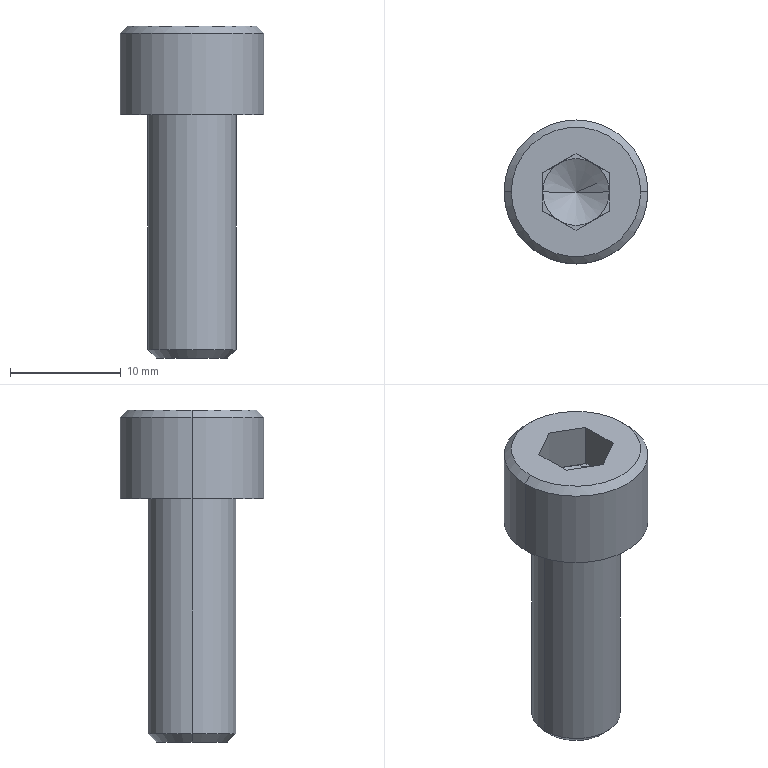Part | NX | features BREP 1 | 1 solid | 25 faces | box 13 x 13 x 30 mm | volume 2011 mm3 | plane 15 | cone 6 | cylinder 4 | commonest cylinder face diameters 8 x2 13 x2
STEP:
#1=CARTESIAN_POINT('',(0.,0.,2.268));
#2=VERTEX_POINT('',#1);
#3=CARTESIAN_POINT('',(3.,0.,4.));
#4=VERTEX_POINT('',#3);
#5=CARTESIAN_POINT('',(0.,0.,2.268));
#6=DIRECTION('',(0.866,0.,0.5));
#7=VECTOR('',#6,1000.);
#8=LINE('',#5,#7);
#9=EDGE_CURVE('',#2,#4,#8,.T.);
#10=ORIENTED_EDGE('',*,*,#9,.F.);
#11=CARTESIAN_POINT('',(-3.,0.,4.));
#12=VERTEX_POINT('',#11);
#13=CARTESIAN_POINT('',(0.,0.,2.268));
#14=DIRECTION('',(-0.866,0.,0.5));
#15=VECTOR('',#14,1000.);
#16=LINE('',#13,#15);
#17=EDGE_CURVE('',#2,#12,#16,.T.);
#18=ORIENTED_EDGE('',*,*,#17,.T.);
#19=CARTESIAN_POINT('',(-1.5,-2.598,4.));
#20=VERTEX_POINT('',#19);
#21=CARTESIAN_POINT('',(0.,0.,4.));
#22=DIRECTION('',(0.,0.,1.));
#23=DIRECTION('',(1.,0.,0.));
#24=AXIS2_PLACEMENT_3D('',#21,#22,#23);
#25=CIRCLE('',#24,3.);
#26=EDGE_CURVE('',#12,#20,#25,.T.);
#27=ORIENTED_EDGE('',*,*,#26,.T.);
#28=CARTESIAN_POINT('',(1.5,-2.598,4.));
#29=VERTEX_POINT('',#28);
#30=CARTESIAN_POINT('',(0.,0.,4.));
#31=DIRECTION('',(0.,0.,1.));
#32=DIRECTION('',(1.,0.,0.));
#33=AXIS2_PLACEMENT_3D('',#30,#31,#32);
#34=CIRCLE('',#33,3.);
#35=EDGE_CURVE('',#20,#29,#34,.T.);
#36=ORIENTED_EDGE('',*,*,#35,.T.);
#37=CARTESIAN_POINT('',(0.,0.,4.));
#38=DIRECTION('',(0.,0.,1.));
#39=DIRECTION('',(1.,0.,0.));
#40=AXIS2_PLACEMENT_3D('',#37,#38,#39);
#41=CIRCLE('',#40,3.);
#42=EDGE_CURVE('',#29,#4,#41,.T.);
#43=ORIENTED_EDGE('',*,*,#42,.T.);
#44=EDGE_LOOP('',(#10,#18,#27,#36,#43));
#45=FACE_BOUND('',#44,.T.);
#46=CARTESIAN_POINT('',(0.,0.,1002.268));
#47=DIRECTION('',(0.,0.,1.));
#48=DIRECTION('',(-1.,0.,0.));
#49=AXIS2_PLACEMENT_3D('',#46,#47,#48);
#50=CONICAL_SURFACE('',#49,1732.051,1.047);
#51=ADVANCED_FACE('',(#45),#50,.F.);
#52=CARTESIAN_POINT('',(6.5,0.,0.));
#53=VERTEX_POINT('',#52);
#54=CARTESIAN_POINT('',(-6.5,0.,0.));
#55=VERTEX_POINT('',#54);
#56=CARTESIAN_POINT('',(0.,0.,0.));
#57=DIRECTION('',(0.,0.,1.));
#58=DIRECTION('',(1.,0.,0.));
#59=AXIS2_PLACEMENT_3D('',#56,#57,#58);
#60=CIRCLE('',#59,6.5);
#61=EDGE_CURVE('',#53,#55,#60,.T.);
#62=ORIENTED_EDGE('',*,*,#61,.T.);
#63=CARTESIAN_POINT('',(-6.5,0.,7.35));
#64=VERTEX_POINT('',#63);
#65=CARTESIAN_POINT('',(-6.5,0.,0.));
#66=DIRECTION('',(0.,0.,1.));
#67=VECTOR('',#66,1000.);
#68=LINE('',#65,#67);
#69=EDGE_CURVE('',#55,#64,#68,.T.);
#70=ORIENTED_EDGE('',*,*,#69,.T.);
#71=CARTESIAN_POINT('',(6.5,0.,7.35));
#72=VERTEX_POINT('',#71);
#73=CARTESIAN_POINT('',(0.,0.,7.35));
#74=DIRECTION('',(0.,0.,1.));
#75=DIRECTION('',(1.,0.,0.));
#76=AXIS2_PLACEMENT_3D('',#73,#74,#75);
#77=CIRCLE('',#76,6.5);
#78=EDGE_CURVE('',#72,#64,#77,.T.);
#79=ORIENTED_EDGE('',*,*,#78,.F.);
#80=CARTESIAN_POINT('',(6.5,0.,0.));
#81=DIRECTION('',(0.,0.,1.));
#82=VECTOR('',#81,1000.);
#83=LINE('',#80,#82);
#84=EDGE_CURVE('',#53,#72,#83,.T.);
#85=ORIENTED_EDGE('',*,*,#84,.F.);
#86=EDGE_LOOP('',(#62,#70,#79,#85));
#87=FACE_BOUND('',#86,.T.);
#88=CARTESIAN_POINT('',(0.,0.,0.));
#89=DIRECTION('',(0.,0.,1.));
#90=DIRECTION('',(-1.,0.,0.));
#91=AXIS2_PLACEMENT_3D('',#88,#89,#90);
#92=CYLINDRICAL_SURFACE('',#91,6.5);
#93=ADVANCED_FACE('',(#87),#92,.T.);
#94=CARTESIAN_POINT('',(5.85,0.,8.));
#95=VERTEX_POINT('',#94);
#96=CARTESIAN_POINT('',(-5.85,0.,8.));
#97=VERTEX_POINT('',#96);
#98=CARTESIAN_POINT('',(0.,0.,8.));
#99=DIRECTION('',(0.,0.,1.));
#100=DIRECTION('',(1.,0.,0.));
#101=AXIS2_PLACEMENT_3D('',#98,#99,#100);
#102=CIRCLE('',#101,5.85);
#103=EDGE_CURVE('',#95,#97,#102,.T.);
#104=ORIENTED_EDGE('',*,*,#103,.F.);
#105=CARTESIAN_POINT('',(6.5,0.,7.35));
#106=DIRECTION('',(0.7071,0.,-0.7071));
#107=VECTOR('',#106,1000.);
#108=LINE('',#105,#107);
#109=EDGE_CURVE('',#72,#95,#108,.F.);
#110=ORIENTED_EDGE('',*,*,#109,.F.);
#111=ORIENTED_EDGE('',*,*,#78,.T.);
#112=CARTESIAN_POINT('',(-6.5,0.,7.35));
#113=DIRECTION('',(-0.7071,0.,-0.7071));
#114=VECTOR('',#113,1000.);
#115=LINE('',#112,#114);
#116=EDGE_CURVE('',#64,#97,#115,.F.);
#117=ORIENTED_EDGE('',*,*,#116,.T.);
#118=EDGE_LOOP('',(#104,#110,#111,#117));
#119=FACE_BOUND('',#118,.T.);
#120=CARTESIAN_POINT('',(0.,0.,7.35));
#121=DIRECTION('',(0.,0.,-1.));
#122=DIRECTION('',(1.,0.,0.));
#123=AXIS2_PLACEMENT_3D('',#120,#121,#122);
#124=CONICAL_SURFACE('',#123,6.5,0.7854);
#125=ADVANCED_FACE('',(#119),#124,.T.);
#126=CARTESIAN_POINT('',(3.233,0.,-22.));
#127=VERTEX_POINT('',#126);
#128=CARTESIAN_POINT('',(-3.233,0.,-22.));
#129=VERTEX_POINT('',#128);
#130=CARTESIAN_POINT('',(0.,0.,-22.));
#131=DIRECTION('',(0.,0.,1.));
#132=DIRECTION('',(1.,0.,0.));
#133=AXIS2_PLACEMENT_3D('',#130,#131,#132);
#134=CIRCLE('',#133,3.233);
#135=EDGE_CURVE('',#127,#129,#134,.T.);
#136=ORIENTED_EDGE('',*,*,#135,.T.);
#137=CARTESIAN_POINT('',(-4.,0.,-21.233));
#138=VERTEX_POINT('',#137);
#139=CARTESIAN_POINT('',(-3.233,0.,-22.));
#140=DIRECTION('',(-0.7071,0.,0.7071));
#141=VECTOR('',#140,1000.);
#142=LINE('',#139,#141);
#143=EDGE_CURVE('',#129,#138,#142,.T.);
#144=ORIENTED_EDGE('',*,*,#143,.T.);
#145=CARTESIAN_POINT('',(4.,0.,-21.233));
#146=VERTEX_POINT('',#145);
#147=CARTESIAN_POINT('',(0.,0.,-21.233));
#148=DIRECTION('',(0.,0.,1.));
#149=DIRECTION('',(1.,0.,0.));
#150=AXIS2_PLACEMENT_3D('',#147,#148,#149);
#151=CIRCLE('',#150,4.);
#152=EDGE_CURVE('',#146,#138,#151,.T.);
#153=ORIENTED_EDGE('',*,*,#152,.F.);
#154=CARTESIAN_POINT('',(3.233,0.,-22.));
#155=DIRECTION('',(0.7071,0.,0.7071));
#156=VECTOR('',#155,1000.);
#157=LINE('',#154,#156);
#158=EDGE_CURVE('',#127,#146,#157,.T.);
#159=ORIENTED_EDGE('',*,*,#158,.F.);
#160=EDGE_LOOP('',(#136,#144,#153,#159));
#161=FACE_BOUND('',#160,.T.);
#162=CARTESIAN_POINT('',(0.,0.,-22.));
#163=DIRECTION('',(0.,0.,1.));
#164=DIRECTION('',(-1.,0.,0.));
#165=AXIS2_PLACEMENT_3D('',#162,#163,#164);
#166=CONICAL_SURFACE('',#165,3.233,0.7854);
#167=ADVANCED_FACE('',(#161),#166,.T.);
#168=ORIENTED_EDGE('',*,*,#152,.T.);
#169=CARTESIAN_POINT('',(-4.,0.,0.));
#170=VERTEX_POINT('',#169);
#171=CARTESIAN_POINT('',(-4.,0.,-22.));
#172=DIRECTION('',(0.,0.,1.));
#173=VECTOR('',#172,1000.);
#174=LINE('',#171,#173);
#175=EDGE_CURVE('',#138,#170,#174,.T.);
#176=ORIENTED_EDGE('',*,*,#175,.T.);
#177=CARTESIAN_POINT('',(4.,0.,0.));
#178=VERTEX_POINT('',#177);
#179=CARTESIAN_POINT('',(0.,0.,0.));
#180=DIRECTION('',(0.,0.,1.));
#181=DIRECTION('',(1.,0.,0.));
#182=AXIS2_PLACEMENT_3D('',#179,#180,#181);
#183=CIRCLE('',#182,4.);
#184=EDGE_CURVE('',#178,#170,#183,.T.);
#185=ORIENTED_EDGE('',*,*,#184,.F.);
#186=CARTESIAN_POINT('',(4.,0.,-22.));
#187=DIRECTION('',(0.,0.,1.));
#188=VECTOR('',#187,1000.);
#189=LINE('',#186,#188);
#190=EDGE_CURVE('',#146,#178,#189,.T.);
#191=ORIENTED_EDGE('',*,*,#190,.F.);
#192=EDGE_LOOP('',(#168,#176,#185,#191));
#193=FACE_BOUND('',#192,.T.);
#194=CARTESIAN_POINT('',(0.,0.,-22.));
#195=DIRECTION('',(0.,0.,1.));
#196=DIRECTION('',(-1.,0.,0.));
#197=AXIS2_PLACEMENT_3D('',#194,#195,#196);
#198=CYLINDRICAL_SURFACE('',#197,4.);
#199=ADVANCED_FACE('',(#193),#198,.T.);
#200=CARTESIAN_POINT('',(1.5,2.598,4.));
#201=VERTEX_POINT('',#200);
#202=CARTESIAN_POINT('',(0.,0.,4.));
#203=DIRECTION('',(0.,0.,1.));
#204=DIRECTION('',(1.,0.,0.));
#205=AXIS2_PLACEMENT_3D('',#202,#203,#204);
#206=CIRCLE('',#205,3.);
#207=EDGE_CURVE('',#4,#201,#206,.T.);
#208=ORIENTED_EDGE('',*,*,#207,.F.);
#209=CARTESIAN_POINT('',(3.,1.732,4.));
#210=VERTEX_POINT('',#209);
#211=CARTESIAN_POINT('',(3.,-1.732,4.));
#212=DIRECTION('',(0.,1.,0.));
#213=VECTOR('',#212,1000.);
#214=LINE('',#211,#213);
#215=EDGE_CURVE('',#4,#210,#214,.T.);
#216=ORIENTED_EDGE('',*,*,#215,.T.);
#217=CARTESIAN_POINT('',(3.,1.732,4.));
#218=DIRECTION('',(-0.866,0.5,0.));
#219=VECTOR('',#218,1000.);
#220=LINE('',#217,#219);
#221=EDGE_CURVE('',#210,#201,#220,.T.);
#222=ORIENTED_EDGE('',*,*,#221,.T.);
#223=EDGE_LOOP('',(#208,#216,#222));
#224=FACE_BOUND('',#223,.T.);
#225=CARTESIAN_POINT('',(0.,0.,4.));
#226=DIRECTION('',(0.,0.,1.));
#227=DIRECTION('',(-1.,0.,0.));
#228=AXIS2_PLACEMENT_3D('',#225,#226,#227);
#229=PLANE('',#228);
#230=ADVANCED_FACE('',(#224),#229,.T.);
#231=CARTESIAN_POINT('',(-1.5,2.598,4.));
#232=VERTEX_POINT('',#231);
#233=CARTESIAN_POINT('',(0.,0.,4.));
#234=DIRECTION('',(0.,0.,1.));
#235=DIRECTION('',(1.,0.,0.));
#236=AXIS2_PLACEMENT_3D('',#233,#234,#235);
#237=CIRCLE('',#236,3.);
#238=EDGE_CURVE('',#201,#232,#237,.T.);
#239=ORIENTED_EDGE('',*,*,#238,.F.);
#240=CARTESIAN_POINT('',(0.,3.464,4.));
#241=VERTEX_POINT('',#240);
#242=CARTESIAN_POINT('',(3.,1.732,4.));
#243=DIRECTION('',(-0.866,0.5,0.));
#244=VECTOR('',#243,1000.);
#245=LINE('',#242,#244);
#246=EDGE_CURVE('',#201,#241,#245,.T.);
#247=ORIENTED_EDGE('',*,*,#246,.T.);
#248=CARTESIAN_POINT('',(0.,3.464,4.));
#249=DIRECTION('',(-0.866,-0.5,0.));
#250=VECTOR('',#249,1000.);
#251=LINE('',#248,#250);
#252=EDGE_CURVE('',#241,#232,#251,.T.);
#253=ORIENTED_EDGE('',*,*,#252,.T.);
#254=EDGE_LOOP('',(#239,#247,#253));
#255=FACE_BOUND('',#254,.T.);
#256=CARTESIAN_POINT('',(0.,0.,4.));
#257=DIRECTION('',(0.,0.,1.));
#258=DIRECTION('',(-1.,0.,0.));
#259=AXIS2_PLACEMENT_3D('',#256,#257,#258);
#260=PLANE('',#259);
#261=ADVANCED_FACE('',(#255),#260,.T.);
#262=CARTESIAN_POINT('',(0.,0.,4.));
#263=DIRECTION('',(0.,0.,1.));
#264=DIRECTION('',(1.,0.,0.));
#265=AXIS2_PLACEMENT_3D('',#262,#263,#264);
#266=CIRCLE('',#265,3.);
#267=EDGE_CURVE('',#232,#12,#266,.T.);
#268=ORIENTED_EDGE('',*,*,#267,.F.);
#269=CARTESIAN_POINT('',(-3.,1.732,4.));
#270=VERTEX_POINT('',#269);
#271=CARTESIAN_POINT('',(0.,3.464,4.));
#272=DIRECTION('',(-0.866,-0.5,0.));
#273=VECTOR('',#272,1000.);
#274=LINE('',#271,#273);
#275=EDGE_CURVE('',#232,#270,#274,.T.);
#276=ORIENTED_EDGE('',*,*,#275,.T.);
#277=CARTESIAN_POINT('',(-3.,1.732,4.));
#278=DIRECTION('',(0.,-1.,0.));
#279=VECTOR('',#278,1000.);
#280=LINE('',#277,#279);
#281=EDGE_CURVE('',#270,#12,#280,.T.);
#282=ORIENTED_EDGE('',*,*,#281,.T.);
#283=EDGE_LOOP('',(#268,#276,#282));
#284=FACE_BOUND('',#283,.T.);
#285=CARTESIAN_POINT('',(0.,0.,4.));
#286=DIRECTION('',(0.,0.,1.));
#287=DIRECTION('',(-1.,0.,0.));
#288=AXIS2_PLACEMENT_3D('',#285,#286,#287);
#289=PLANE('',#288);
#290=ADVANCED_FACE('',(#284),#289,.T.);
#291=ORIENTED_EDGE('',*,*,#26,.F.);
#292=CARTESIAN_POINT('',(-3.,-1.732,4.));
#293=VERTEX_POINT('',#292);
#294=CARTESIAN_POINT('',(-3.,1.732,4.));
#295=DIRECTION('',(0.,-1.,0.));
#296=VECTOR('',#295,1000.);
#297=LINE('',#294,#296);
#298=EDGE_CURVE('',#12,#293,#297,.T.);
#299=ORIENTED_EDGE('',*,*,#298,.T.);
#300=CARTESIAN_POINT('',(-3.,-1.732,4.));
#301=DIRECTION('',(0.866,-0.5,0.));
#302=VECTOR('',#301,1000.);
#303=LINE('',#300,#302);
#304=EDGE_CURVE('',#293,#20,#303,.T.);
#305=ORIENTED_EDGE('',*,*,#304,.T.);
#306=EDGE_LOOP('',(#291,#299,#305));
#307=FACE_BOUND('',#306,.T.);
#308=CARTESIAN_POINT('',(0.,0.,4.));
#309=DIRECTION('',(0.,0.,1.));
#310=DIRECTION('',(-1.,0.,0.));
#311=AXIS2_PLACEMENT_3D('',#308,#309,#310);
#312=PLANE('',#311);
#313=ADVANCED_FACE('',(#307),#312,.T.);
#314=ORIENTED_EDGE('',*,*,#35,.F.);
#315=CARTESIAN_POINT('',(0.,-3.464,4.));
#316=VERTEX_POINT('',#315);
#317=CARTESIAN_POINT('',(-3.,-1.732,4.));
#318=DIRECTION('',(0.866,-0.5,0.));
#319=VECTOR('',#318,1000.);
#320=LINE('',#317,#319);
#321=EDGE_CURVE('',#20,#316,#320,.T.);
#322=ORIENTED_EDGE('',*,*,#321,.T.);
#323=CARTESIAN_POINT('',(0.,-3.464,4.));
#324=DIRECTION('',(0.866,0.5,0.));
#325=VECTOR('',#324,1000.);
#326=LINE('',#323,#325);
#327=EDGE_CURVE('',#316,#29,#326,.T.);
#328=ORIENTED_EDGE('',*,*,#327,.T.);
#329=EDGE_LOOP('',(#314,#322,#328));
#330=FACE_BOUND('',#329,.T.);
#331=CARTESIAN_POINT('',(0.,0.,4.));
#332=DIRECTION('',(0.,0.,1.));
#333=DIRECTION('',(-1.,0.,0.));
#334=AXIS2_PLACEMENT_3D('',#331,#332,#333);
#335=PLANE('',#334);
#336=ADVANCED_FACE('',(#330),#335,.T.);
#337=ORIENTED_EDGE('',*,*,#175,.F.);
#338=CARTESIAN_POINT('',(0.,0.,-21.233));
#339=DIRECTION('',(0.,0.,1.));
#340=DIRECTION('',(1.,0.,0.));
#341=AXIS2_PLACEMENT_3D('',#338,#339,#340);
#342=CIRCLE('',#341,4.);
#343=EDGE_CURVE('',#138,#146,#342,.T.);
#344=ORIENTED_EDGE('',*,*,#343,.T.);
#345=ORIENTED_EDGE('',*,*,#190,.T.);
#346=CARTESIAN_POINT('',(0.,0.,0.));
#347=DIRECTION('',(0.,0.,1.));
#348=DIRECTION('',(1.,0.,0.));
#349=AXIS2_PLACEMENT_3D('',#346,#347,#348);
#350=CIRCLE('',#349,4.);
#351=EDGE_CURVE('',#170,#178,#350,.T.);
#352=ORIENTED_EDGE('',*,*,#351,.F.);
#353=EDGE_LOOP('',(#337,#344,#345,#352));
#354=FACE_BOUND('',#353,.T.);
#355=CARTESIAN_POINT('',(0.,0.,-22.));
#356=DIRECTION('',(0.,0.,1.));
#357=DIRECTION('',(-1.,0.,0.));
#358=AXIS2_PLACEMENT_3D('',#355,#356,#357);
#359=CYLINDRICAL_SURFACE('',#358,4.);
#360=ADVANCED_FACE('',(#354),#359,.T.);
#361=ORIENTED_EDGE('',*,*,#143,.F.);
#362=CARTESIAN_POINT('',(0.,0.,-22.));
#363=DIRECTION('',(0.,0.,1.));
#364=DIRECTION('',(1.,0.,0.));
#365=AXIS2_PLACEMENT_3D('',#362,#363,#364);
#366=CIRCLE('',#365,3.233);
#367=EDGE_CURVE('',#129,#127,#366,.T.);
#368=ORIENTED_EDGE('',*,*,#367,.T.);
#369=ORIENTED_EDGE('',*,*,#158,.T.);
#370=ORIENTED_EDGE('',*,*,#343,.F.);
#371=EDGE_LOOP('',(#361,#368,#369,#370));
#372=FACE_BOUND('',#371,.T.);
#373=CARTESIAN_POINT('',(0.,0.,-22.));
#374=DIRECTION('',(0.,0.,1.));
#375=DIRECTION('',(-1.,0.,0.));
#376=AXIS2_PLACEMENT_3D('',#373,#374,#375);
#377=CONICAL_SURFACE('',#376,3.233,0.7854);
#378=ADVANCED_FACE('',(#372),#377,.T.);
#379=ORIENTED_EDGE('',*,*,#135,.F.);
#380=ORIENTED_EDGE('',*,*,#367,.F.);
#381=EDGE_LOOP('',(#379,#380));
#382=FACE_BOUND('',#381,.T.);
#383=CARTESIAN_POINT('',(0.,3.233,-22.));
#384=DIRECTION('',(0.,0.,1.));
#385=DIRECTION('',(-1.,0.,0.));
#386=AXIS2_PLACEMENT_3D('',#383,#384,#385);
#387=PLANE('',#386);
#388=ADVANCED_FACE('',(#382),#387,.F.);
#389=CARTESIAN_POINT('',(0.,-3.464,8.));
#390=VERTEX_POINT('',#389);
#391=CARTESIAN_POINT('',(3.,-1.732,8.));
#392=VERTEX_POINT('',#391);
#393=CARTESIAN_POINT('',(0.,-3.464,8.));
#394=DIRECTION('',(0.866,0.5,0.));
#395=VECTOR('',#394,1000.);
#396=LINE('',#393,#395);
#397=EDGE_CURVE('',#390,#392,#396,.T.);
#398=ORIENTED_EDGE('',*,*,#397,.F.);
#399=CARTESIAN_POINT('',(-3.,-1.732,8.));
#400=VERTEX_POINT('',#399);
#401=CARTESIAN_POINT('',(-3.,-1.732,8.));
#402=DIRECTION('',(0.866,-0.5,0.));
#403=VECTOR('',#402,1000.);
#404=LINE('',#401,#403);
#405=EDGE_CURVE('',#400,#390,#404,.T.);
#406=ORIENTED_EDGE('',*,*,#405,.F.);
#407=CARTESIAN_POINT('',(-3.,1.732,8.));
#408=VERTEX_POINT('',#407);
#409=CARTESIAN_POINT('',(-3.,1.732,8.));
#410=DIRECTION('',(0.,-1.,0.));
#411=VECTOR('',#410,1000.);
#412=LINE('',#409,#411);
#413=EDGE_CURVE('',#408,#400,#412,.T.);
#414=ORIENTED_EDGE('',*,*,#413,.F.);
#415=CARTESIAN_POINT('',(0.,3.464,8.));
#416=VERTEX_POINT('',#415);
#417=CARTESIAN_POINT('',(0.,3.464,8.));
#418=DIRECTION('',(-0.866,-0.5,0.));
#419=VECTOR('',#418,1000.);
#420=LINE('',#417,#419);
#421=EDGE_CURVE('',#416,#408,#420,.T.);
#422=ORIENTED_EDGE('',*,*,#421,.F.);
#423=CARTESIAN_POINT('',(3.,1.732,8.));
#424=VERTEX_POINT('',#423);
#425=CARTESIAN_POINT('',(3.,1.732,8.));
#426=DIRECTION('',(-0.866,0.5,0.));
#427=VECTOR('',#426,1000.);
#428=LINE('',#425,#427);
#429=EDGE_CURVE('',#424,#416,#428,.T.);
#430=ORIENTED_EDGE('',*,*,#429,.F.);
#431=CARTESIAN_POINT('',(3.,-1.732,8.));
#432=DIRECTION('',(0.,1.,0.));
#433=VECTOR('',#432,1000.);
#434=LINE('',#431,#433);
#435=EDGE_CURVE('',#392,#424,#434,.T.);
#436=ORIENTED_EDGE('',*,*,#435,.F.);
#437=EDGE_LOOP('',(#398,#406,#414,#422,#430,#436));
#438=FACE_BOUND('',#437,.T.);
#439=CARTESIAN_POINT('',(0.,0.,8.));
#440=DIRECTION('',(0.,0.,1.));
#441=DIRECTION('',(1.,0.,0.));
#442=AXIS2_PLACEMENT_3D('',#439,#440,#441);
#443=CIRCLE('',#442,5.85);
#444=EDGE_CURVE('',#97,#95,#443,.T.);
#445=ORIENTED_EDGE('',*,*,#444,.T.);
#446=ORIENTED_EDGE('',*,*,#103,.T.);
#447=EDGE_LOOP('',(#445,#446));
#448=FACE_BOUND('',#447,.T.);
#449=CARTESIAN_POINT('',(0.,0.,8.));
#450=DIRECTION('',(0.,0.,-1.));
#451=DIRECTION('',(1.,0.,0.));
#452=AXIS2_PLACEMENT_3D('',#449,#450,#451);
#453=PLANE('',#452);
#454=ADVANCED_FACE('',(#438,#448),#453,.F.);
#455=ORIENTED_EDGE('',*,*,#109,.T.);
#456=ORIENTED_EDGE('',*,*,#444,.F.);
#457=ORIENTED_EDGE('',*,*,#116,.F.);
#458=CARTESIAN_POINT('',(0.,0.,7.35));
#459=DIRECTION('',(0.,0.,1.));
#460=DIRECTION('',(1.,0.,0.));
#461=AXIS2_PLACEMENT_3D('',#458,#459,#460);
#462=CIRCLE('',#461,6.5);
#463=EDGE_CURVE('',#64,#72,#462,.T.);
#464=ORIENTED_EDGE('',*,*,#463,.T.);
#465=EDGE_LOOP('',(#455,#456,#457,#464));
#466=FACE_BOUND('',#465,.T.);
#467=CARTESIAN_POINT('',(0.,0.,7.35));
#468=DIRECTION('',(0.,0.,-1.));
#469=DIRECTION('',(1.,0.,0.));
#470=AXIS2_PLACEMENT_3D('',#467,#468,#469);
#471=CONICAL_SURFACE('',#470,6.5,0.7854);
#472=ADVANCED_FACE('',(#466),#471,.T.);
#473=ORIENTED_EDGE('',*,*,#69,.F.);
#474=CARTESIAN_POINT('',(0.,0.,0.));
#475=DIRECTION('',(0.,0.,1.));
#476=DIRECTION('',(1.,0.,0.));
#477=AXIS2_PLACEMENT_3D('',#474,#475,#476);
#478=CIRCLE('',#477,6.5);
#479=EDGE_CURVE('',#55,#53,#478,.T.);
#480=ORIENTED_EDGE('',*,*,#479,.T.);
#481=ORIENTED_EDGE('',*,*,#84,.T.);
#482=ORIENTED_EDGE('',*,*,#463,.F.);
#483=EDGE_LOOP('',(#473,#480,#481,#482));
#484=FACE_BOUND('',#483,.T.);
#485=CARTESIAN_POINT('',(0.,0.,0.));
#486=DIRECTION('',(0.,0.,1.));
#487=DIRECTION('',(-1.,0.,0.));
#488=AXIS2_PLACEMENT_3D('',#485,#486,#487);
#489=CYLINDRICAL_SURFACE('',#488,6.5);
#490=ADVANCED_FACE('',(#484),#489,.T.);
#491=ORIENTED_EDGE('',*,*,#184,.T.);
#492=ORIENTED_EDGE('',*,*,#351,.T.);
#493=EDGE_LOOP('',(#491,#492));
#494=FACE_BOUND('',#493,.T.);
#495=ORIENTED_EDGE('',*,*,#61,.F.);
#496=ORIENTED_EDGE('',*,*,#479,.F.);
#497=EDGE_LOOP('',(#495,#496));
#498=FACE_BOUND('',#497,.T.);
#499=CARTESIAN_POINT('',(0.,6.5,0.));
#500=DIRECTION('',(0.,0.,1.));
#501=DIRECTION('',(-1.,0.,0.));
#502=AXIS2_PLACEMENT_3D('',#499,#500,#501);
#503=PLANE('',#502);
#504=ADVANCED_FACE('',(#494,#498),#503,.F.);
#505=ORIENTED_EDGE('',*,*,#405,.T.);
#506=CARTESIAN_POINT('',(0.,-3.464,4.));
#507=DIRECTION('',(0.,0.,1.));
#508=VECTOR('',#507,1000.);
#509=LINE('',#506,#508);
#510=EDGE_CURVE('',#316,#390,#509,.T.);
#511=ORIENTED_EDGE('',*,*,#510,.F.);
#512=ORIENTED_EDGE('',*,*,#321,.F.);
#513=ORIENTED_EDGE('',*,*,#304,.F.);
#514=CARTESIAN_POINT('',(-3.,-1.732,4.));
#515=DIRECTION('',(0.,0.,1.));
#516=VECTOR('',#515,1000.);
#517=LINE('',#514,#516);
#518=EDGE_CURVE('',#293,#400,#517,.T.);
#519=ORIENTED_EDGE('',*,*,#518,.T.);
#520=EDGE_LOOP('',(#505,#511,#512,#513,#519));
#521=FACE_BOUND('',#520,.T.);
#522=CARTESIAN_POINT('',(-3.,-1.732,4.));
#523=DIRECTION('',(-0.5,-0.866,0.));
#524=DIRECTION('',(-0.866,0.5,0.));
#525=AXIS2_PLACEMENT_3D('',#522,#523,#524);
#526=PLANE('',#525);
#527=ADVANCED_FACE('',(#521),#526,.F.);
#528=ORIENTED_EDGE('',*,*,#413,.T.);
#529=ORIENTED_EDGE('',*,*,#518,.F.);
#530=ORIENTED_EDGE('',*,*,#298,.F.);
#531=ORIENTED_EDGE('',*,*,#281,.F.);
#532=CARTESIAN_POINT('',(-3.,1.732,4.));
#533=DIRECTION('',(0.,0.,1.));
#534=VECTOR('',#533,1000.);
#535=LINE('',#532,#534);
#536=EDGE_CURVE('',#270,#408,#535,.T.);
#537=ORIENTED_EDGE('',*,*,#536,.T.);
#538=EDGE_LOOP('',(#528,#529,#530,#531,#537));
#539=FACE_BOUND('',#538,.T.);
#540=CARTESIAN_POINT('',(-3.,1.732,4.));
#541=DIRECTION('',(-1.,0.,0.));
#542=DIRECTION('',(0.,0.,-1.));
#543=AXIS2_PLACEMENT_3D('',#540,#541,#542);
#544=PLANE('',#543);
#545=ADVANCED_FACE('',(#539),#544,.F.);
#546=ORIENTED_EDGE('',*,*,#421,.T.);
#547=ORIENTED_EDGE('',*,*,#536,.F.);
#548=ORIENTED_EDGE('',*,*,#275,.F.);
#549=ORIENTED_EDGE('',*,*,#252,.F.);
#550=CARTESIAN_POINT('',(0.,3.464,4.));
#551=DIRECTION('',(0.,0.,1.));
#552=VECTOR('',#551,1000.);
#553=LINE('',#550,#552);
#554=EDGE_CURVE('',#241,#416,#553,.T.);
#555=ORIENTED_EDGE('',*,*,#554,.T.);
#556=EDGE_LOOP('',(#546,#547,#548,#549,#555));
#557=FACE_BOUND('',#556,.T.);
#558=CARTESIAN_POINT('',(0.,3.464,4.));
#559=DIRECTION('',(-0.5,0.866,0.));
#560=DIRECTION('',(0.866,0.5,0.));
#561=AXIS2_PLACEMENT_3D('',#558,#559,#560);
#562=PLANE('',#561);
#563=ADVANCED_FACE('',(#557),#562,.F.);
#564=ORIENTED_EDGE('',*,*,#429,.T.);
#565=ORIENTED_EDGE('',*,*,#554,.F.);
#566=ORIENTED_EDGE('',*,*,#246,.F.);
#567=ORIENTED_EDGE('',*,*,#221,.F.);
#568=CARTESIAN_POINT('',(3.,1.732,4.));
#569=DIRECTION('',(0.,0.,1.));
#570=VECTOR('',#569,1000.);
#571=LINE('',#568,#570);
#572=EDGE_CURVE('',#210,#424,#571,.T.);
#573=ORIENTED_EDGE('',*,*,#572,.T.);
#574=EDGE_LOOP('',(#564,#565,#566,#567,#573));
#575=FACE_BOUND('',#574,.T.);
#576=CARTESIAN_POINT('',(3.,1.732,4.));
#577=DIRECTION('',(0.5,0.866,0.));
#578=DIRECTION('',(0.866,-0.5,0.));
#579=AXIS2_PLACEMENT_3D('',#576,#577,#578);
#580=PLANE('',#579);
#581=ADVANCED_FACE('',(#575),#580,.F.);
#582=ORIENTED_EDGE('',*,*,#435,.T.);
#583=ORIENTED_EDGE('',*,*,#572,.F.);
#584=ORIENTED_EDGE('',*,*,#215,.F.);
#585=CARTESIAN_POINT('',(3.,-1.732,4.));
#586=VERTEX_POINT('',#585);
#587=CARTESIAN_POINT('',(3.,-1.732,4.));
#588=DIRECTION('',(0.,1.,0.));
#589=VECTOR('',#588,1000.);
#590=LINE('',#587,#589);
#591=EDGE_CURVE('',#586,#4,#590,.T.);
#592=ORIENTED_EDGE('',*,*,#591,.F.);
#593=CARTESIAN_POINT('',(3.,-1.732,4.));
#594=DIRECTION('',(0.,0.,1.));
#595=VECTOR('',#594,1000.);
#596=LINE('',#593,#595);
#597=EDGE_CURVE('',#586,#392,#596,.T.);
#598=ORIENTED_EDGE('',*,*,#597,.T.);
#599=EDGE_LOOP('',(#582,#583,#584,#592,#598));
#600=FACE_BOUND('',#599,.T.);
#601=CARTESIAN_POINT('',(3.,-1.732,4.));
#602=DIRECTION('',(1.,0.,0.));
#603=DIRECTION('',(0.,0.,1.));
#604=AXIS2_PLACEMENT_3D('',#601,#602,#603);
#605=PLANE('',#604);
#606=ADVANCED_FACE('',(#600),#605,.F.);
#607=ORIENTED_EDGE('',*,*,#397,.T.);
#608=ORIENTED_EDGE('',*,*,#597,.F.);
#609=CARTESIAN_POINT('',(0.,-3.464,4.));
#610=DIRECTION('',(0.866,0.5,0.));
#611=VECTOR('',#610,1000.);
#612=LINE('',#609,#611);
#613=EDGE_CURVE('',#29,#586,#612,.T.);
#614=ORIENTED_EDGE('',*,*,#613,.F.);
#615=ORIENTED_EDGE('',*,*,#327,.F.);
#616=ORIENTED_EDGE('',*,*,#510,.T.);
#617=EDGE_LOOP('',(#607,#608,#614,#615,#616));
#618=FACE_BOUND('',#617,.T.);
#619=CARTESIAN_POINT('',(0.,-3.464,4.));
#620=DIRECTION('',(0.5,-0.866,0.));
#621=DIRECTION('',(-0.866,-0.5,0.));
#622=AXIS2_PLACEMENT_3D('',#619,#620,#621);
#623=PLANE('',#622);
#624=ADVANCED_FACE('',(#618),#623,.F.);
#625=ORIENTED_EDGE('',*,*,#42,.F.);
#626=ORIENTED_EDGE('',*,*,#613,.T.);
#627=ORIENTED_EDGE('',*,*,#591,.T.);
#628=EDGE_LOOP('',(#625,#626,#627));
#629=FACE_BOUND('',#628,.T.);
#630=CARTESIAN_POINT('',(0.,0.,4.));
#631=DIRECTION('',(0.,0.,1.));
#632=DIRECTION('',(-1.,0.,0.));
#633=AXIS2_PLACEMENT_3D('',#630,#631,#632);
#634=PLANE('',#633);
#635=ADVANCED_FACE('',(#629),#634,.T.);
#636=ORIENTED_EDGE('',*,*,#17,.F.);
#637=ORIENTED_EDGE('',*,*,#9,.T.);
#638=ORIENTED_EDGE('',*,*,#207,.T.);
#639=ORIENTED_EDGE('',*,*,#238,.T.);
#640=ORIENTED_EDGE('',*,*,#267,.T.);
#641=EDGE_LOOP('',(#636,#637,#638,#639,#640));
#642=FACE_BOUND('',#641,.T.);
#643=CARTESIAN_POINT('',(0.,0.,1002.268));
#644=DIRECTION('',(0.,0.,1.));
#645=DIRECTION('',(-1.,0.,0.));
#646=AXIS2_PLACEMENT_3D('',#643,#644,#645);
#647=CONICAL_SURFACE('',#646,1732.051,1.047);
#648=ADVANCED_FACE('',(#642),#647,.F.);
#649=CLOSED_SHELL('',(#51,#93,#125,#167,#199,#230,#261,#290,#313,#336,#360,#378,#388,#454,#472,#490,#504,#527,#545,#563,#581,#606,#624,#635,#648));
#650=MANIFOLD_SOLID_BREP('',#649);
#651=(LENGTH_UNIT()NAMED_UNIT(*)SI_UNIT(.MILLI.,.METRE.));
#652=UNCERTAINTY_MEASURE_WITH_UNIT(LENGTH_MEASURE(0.00001),#651,'','');
#653=(NAMED_UNIT(*)PLANE_ANGLE_UNIT()SI_UNIT($,.RADIAN.));
#654=(NAMED_UNIT(*)SI_UNIT($,.STERADIAN.)SOLID_ANGLE_UNIT());
#655=(GEOMETRIC_REPRESENTATION_CONTEXT(3)GLOBAL_UNCERTAINTY_ASSIGNED_CONTEXT((#652))GLOBAL_UNIT_ASSIGNED_CONTEXT((#651,#653,#654))REPRESENTATION_CONTEXT('',''));
#656=ADVANCED_BREP_SHAPE_REPRESENTATION('',(#650),#655);